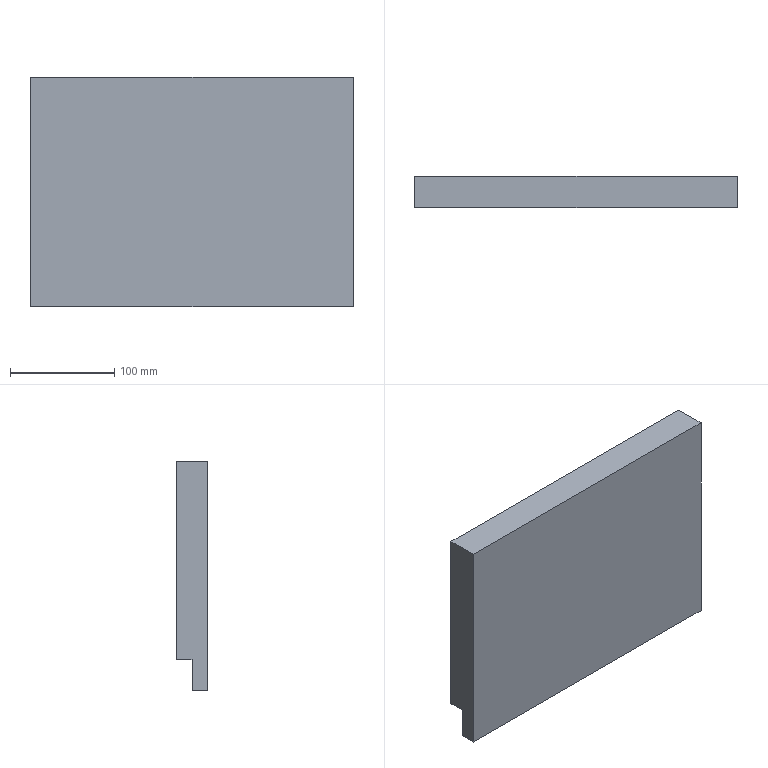Part | SolidWorks | features Cut 1, Extrusion 1 | 1 solid | 8 faces | box 308.5 x 30 x 220 mm | volume 1897275 mm3 | plane 8
STEP:
#1=CARTESIAN_POINT('',(154.25,15.,-110.));
#2=VERTEX_POINT('',#1);
#3=CARTESIAN_POINT('',(154.25,15.,-80.));
#4=VERTEX_POINT('',#3);
#5=CARTESIAN_POINT('',(154.25,15.,110.));
#6=DIRECTION('',(0.,0.,1.));
#7=VECTOR('',#6,1000.);
#8=LINE('',#5,#7);
#9=EDGE_CURVE('',#2,#4,#8,.T.);
#10=ORIENTED_EDGE('',*,*,#9,.T.);
#11=CARTESIAN_POINT('',(154.25,30.,-80.));
#12=VERTEX_POINT('',#11);
#13=CARTESIAN_POINT('',(154.25,30.,-80.));
#14=DIRECTION('',(0.,1.,0.));
#15=VECTOR('',#14,1000.);
#16=LINE('',#13,#15);
#17=EDGE_CURVE('',#4,#12,#16,.T.);
#18=ORIENTED_EDGE('',*,*,#17,.T.);
#19=CARTESIAN_POINT('',(154.25,30.,110.));
#20=VERTEX_POINT('',#19);
#21=CARTESIAN_POINT('',(154.25,30.,110.));
#22=DIRECTION('',(0.,0.,-1.));
#23=VECTOR('',#22,1000.);
#24=LINE('',#21,#23);
#25=EDGE_CURVE('',#20,#12,#24,.T.);
#26=ORIENTED_EDGE('',*,*,#25,.F.);
#27=CARTESIAN_POINT('',(154.25,0.,110.));
#28=VERTEX_POINT('',#27);
#29=CARTESIAN_POINT('',(154.25,30.,110.));
#30=DIRECTION('',(0.,-1.,0.));
#31=VECTOR('',#30,1000.);
#32=LINE('',#29,#31);
#33=EDGE_CURVE('',#20,#28,#32,.T.);
#34=ORIENTED_EDGE('',*,*,#33,.T.);
#35=CARTESIAN_POINT('',(154.25,0.,-110.));
#36=VERTEX_POINT('',#35);
#37=CARTESIAN_POINT('',(154.25,0.,110.));
#38=DIRECTION('',(0.,0.,-1.));
#39=VECTOR('',#38,1000.);
#40=LINE('',#37,#39);
#41=EDGE_CURVE('',#28,#36,#40,.T.);
#42=ORIENTED_EDGE('',*,*,#41,.T.);
#43=CARTESIAN_POINT('',(154.25,30.,-110.));
#44=DIRECTION('',(0.,-1.,0.));
#45=VECTOR('',#44,1000.);
#46=LINE('',#43,#45);
#47=EDGE_CURVE('',#2,#36,#46,.T.);
#48=ORIENTED_EDGE('',*,*,#47,.F.);
#49=EDGE_LOOP('',(#10,#18,#26,#34,#42,#48));
#50=FACE_OUTER_BOUND('',#49,.T.);
#51=CARTESIAN_POINT('',(154.25,30.,110.));
#52=DIRECTION('',(-1.,0.,0.));
#53=DIRECTION('',(0.,0.,1.));
#54=AXIS2_PLACEMENT_3D('',#51,#52,#53);
#55=PLANE('',#54);
#56=ADVANCED_FACE('',(#50),#55,.F.);
#57=CARTESIAN_POINT('',(-154.25,15.,-110.));
#58=VERTEX_POINT('',#57);
#59=CARTESIAN_POINT('',(-154.25,0.,-110.));
#60=VERTEX_POINT('',#59);
#61=CARTESIAN_POINT('',(-154.25,30.,-110.));
#62=DIRECTION('',(0.,-1.,0.));
#63=VECTOR('',#62,1000.);
#64=LINE('',#61,#63);
#65=EDGE_CURVE('',#58,#60,#64,.T.);
#66=ORIENTED_EDGE('',*,*,#65,.F.);
#67=CARTESIAN_POINT('',(-154.25,15.,-110.));
#68=DIRECTION('',(1.,0.,0.));
#69=VECTOR('',#68,1000.);
#70=LINE('',#67,#69);
#71=EDGE_CURVE('',#58,#2,#70,.T.);
#72=ORIENTED_EDGE('',*,*,#71,.T.);
#73=ORIENTED_EDGE('',*,*,#47,.T.);
#74=CARTESIAN_POINT('',(-154.25,0.,-110.));
#75=DIRECTION('',(-1.,0.,0.));
#76=VECTOR('',#75,1000.);
#77=LINE('',#74,#76);
#78=EDGE_CURVE('',#36,#60,#77,.T.);
#79=ORIENTED_EDGE('',*,*,#78,.T.);
#80=EDGE_LOOP('',(#66,#72,#73,#79));
#81=FACE_OUTER_BOUND('',#80,.T.);
#82=CARTESIAN_POINT('',(-154.25,30.,-110.));
#83=DIRECTION('',(0.,0.,1.));
#84=DIRECTION('',(1.,0.,0.));
#85=AXIS2_PLACEMENT_3D('',#82,#83,#84);
#86=PLANE('',#85);
#87=ADVANCED_FACE('',(#81),#86,.F.);
#88=CARTESIAN_POINT('',(-154.25,30.,-80.));
#89=VERTEX_POINT('',#88);
#90=CARTESIAN_POINT('',(-154.25,30.,110.));
#91=VERTEX_POINT('',#90);
#92=CARTESIAN_POINT('',(-154.25,30.,110.));
#93=DIRECTION('',(0.,0.,1.));
#94=VECTOR('',#93,1000.);
#95=LINE('',#92,#94);
#96=EDGE_CURVE('',#89,#91,#95,.T.);
#97=ORIENTED_EDGE('',*,*,#96,.F.);
#98=CARTESIAN_POINT('',(-154.25,15.,-80.));
#99=VERTEX_POINT('',#98);
#100=CARTESIAN_POINT('',(-154.25,30.,-80.));
#101=DIRECTION('',(0.,-1.,0.));
#102=VECTOR('',#101,1000.);
#103=LINE('',#100,#102);
#104=EDGE_CURVE('',#89,#99,#103,.T.);
#105=ORIENTED_EDGE('',*,*,#104,.T.);
#106=CARTESIAN_POINT('',(-154.25,15.,110.));
#107=DIRECTION('',(0.,0.,-1.));
#108=VECTOR('',#107,1000.);
#109=LINE('',#106,#108);
#110=EDGE_CURVE('',#99,#58,#109,.T.);
#111=ORIENTED_EDGE('',*,*,#110,.T.);
#112=ORIENTED_EDGE('',*,*,#65,.T.);
#113=CARTESIAN_POINT('',(-154.25,0.,110.));
#114=VERTEX_POINT('',#113);
#115=CARTESIAN_POINT('',(-154.25,0.,110.));
#116=DIRECTION('',(0.,0.,1.));
#117=VECTOR('',#116,1000.);
#118=LINE('',#115,#117);
#119=EDGE_CURVE('',#60,#114,#118,.T.);
#120=ORIENTED_EDGE('',*,*,#119,.T.);
#121=CARTESIAN_POINT('',(-154.25,30.,110.));
#122=DIRECTION('',(0.,-1.,0.));
#123=VECTOR('',#122,1000.);
#124=LINE('',#121,#123);
#125=EDGE_CURVE('',#91,#114,#124,.T.);
#126=ORIENTED_EDGE('',*,*,#125,.F.);
#127=EDGE_LOOP('',(#97,#105,#111,#112,#120,#126));
#128=FACE_OUTER_BOUND('',#127,.T.);
#129=CARTESIAN_POINT('',(-154.25,30.,110.));
#130=DIRECTION('',(1.,0.,0.));
#131=DIRECTION('',(0.,0.,-1.));
#132=AXIS2_PLACEMENT_3D('',#129,#130,#131);
#133=PLANE('',#132);
#134=ADVANCED_FACE('',(#128),#133,.F.);
#135=CARTESIAN_POINT('',(-154.25,0.,110.));
#136=DIRECTION('',(1.,0.,0.));
#137=VECTOR('',#136,1000.);
#138=LINE('',#135,#137);
#139=EDGE_CURVE('',#114,#28,#138,.T.);
#140=ORIENTED_EDGE('',*,*,#139,.T.);
#141=ORIENTED_EDGE('',*,*,#33,.F.);
#142=CARTESIAN_POINT('',(-154.25,30.,110.));
#143=DIRECTION('',(1.,0.,0.));
#144=VECTOR('',#143,1000.);
#145=LINE('',#142,#144);
#146=EDGE_CURVE('',#91,#20,#145,.T.);
#147=ORIENTED_EDGE('',*,*,#146,.F.);
#148=ORIENTED_EDGE('',*,*,#125,.T.);
#149=EDGE_LOOP('',(#140,#141,#147,#148));
#150=FACE_OUTER_BOUND('',#149,.T.);
#151=CARTESIAN_POINT('',(-154.25,30.,110.));
#152=DIRECTION('',(0.,0.,-1.));
#153=DIRECTION('',(-1.,0.,0.));
#154=AXIS2_PLACEMENT_3D('',#151,#152,#153);
#155=PLANE('',#154);
#156=ADVANCED_FACE('',(#150),#155,.F.);
#157=ORIENTED_EDGE('',*,*,#25,.T.);
#158=CARTESIAN_POINT('',(0.,30.,-80.));
#159=DIRECTION('',(-1.,0.,0.));
#160=VECTOR('',#159,1000.);
#161=LINE('',#158,#160);
#162=EDGE_CURVE('',#12,#89,#161,.T.);
#163=ORIENTED_EDGE('',*,*,#162,.T.);
#164=ORIENTED_EDGE('',*,*,#96,.T.);
#165=ORIENTED_EDGE('',*,*,#146,.T.);
#166=EDGE_LOOP('',(#157,#163,#164,#165));
#167=FACE_OUTER_BOUND('',#166,.T.);
#168=CARTESIAN_POINT('',(0.,30.,0.));
#169=DIRECTION('',(0.,-1.,0.));
#170=DIRECTION('',(0.,0.,-1.));
#171=AXIS2_PLACEMENT_3D('',#168,#169,#170);
#172=PLANE('',#171);
#173=ADVANCED_FACE('',(#167),#172,.F.);
#174=ORIENTED_EDGE('',*,*,#41,.F.);
#175=ORIENTED_EDGE('',*,*,#139,.F.);
#176=ORIENTED_EDGE('',*,*,#119,.F.);
#177=ORIENTED_EDGE('',*,*,#78,.F.);
#178=EDGE_LOOP('',(#174,#175,#176,#177));
#179=FACE_OUTER_BOUND('',#178,.T.);
#180=CARTESIAN_POINT('',(0.,0.,0.));
#181=DIRECTION('',(0.,-1.,0.));
#182=DIRECTION('',(0.,0.,-1.));
#183=AXIS2_PLACEMENT_3D('',#180,#181,#182);
#184=PLANE('',#183);
#185=ADVANCED_FACE('',(#179),#184,.T.);
#186=ORIENTED_EDGE('',*,*,#71,.F.);
#187=ORIENTED_EDGE('',*,*,#110,.F.);
#188=CARTESIAN_POINT('',(-167.454,15.,-80.));
#189=DIRECTION('',(1.,0.,0.));
#190=VECTOR('',#189,1000.);
#191=LINE('',#188,#190);
#192=EDGE_CURVE('',#99,#4,#191,.T.);
#193=ORIENTED_EDGE('',*,*,#192,.T.);
#194=ORIENTED_EDGE('',*,*,#9,.F.);
#195=EDGE_LOOP('',(#186,#187,#193,#194));
#196=FACE_OUTER_BOUND('',#195,.T.);
#197=CARTESIAN_POINT('',(0.,15.,0.));
#198=DIRECTION('',(0.,-1.,0.));
#199=DIRECTION('',(0.,0.,-1.));
#200=AXIS2_PLACEMENT_3D('',#197,#198,#199);
#201=PLANE('',#200);
#202=ADVANCED_FACE('',(#196),#201,.F.);
#203=ORIENTED_EDGE('',*,*,#192,.F.);
#204=ORIENTED_EDGE('',*,*,#104,.F.);
#205=ORIENTED_EDGE('',*,*,#162,.F.);
#206=ORIENTED_EDGE('',*,*,#17,.F.);
#207=EDGE_LOOP('',(#203,#204,#205,#206));
#208=FACE_OUTER_BOUND('',#207,.T.);
#209=CARTESIAN_POINT('',(-167.454,15.,-80.));
#210=DIRECTION('',(0.,0.,1.));
#211=DIRECTION('',(1.,0.,0.));
#212=AXIS2_PLACEMENT_3D('',#209,#210,#211);
#213=PLANE('',#212);
#214=ADVANCED_FACE('',(#208),#213,.F.);
#215=CLOSED_SHELL('',(#56,#87,#134,#156,#173,#185,#202,#214));
#216=MANIFOLD_SOLID_BREP('',#215);
#217=CARTESIAN_POINT('',(0.,0.,0.));
#218=DIRECTION('',(0.,0.,1.));
#219=DIRECTION('',(1.,0.,0.));
#220=AXIS2_PLACEMENT_3D('',#217,#218,#219);
#221=(LENGTH_UNIT()NAMED_UNIT(*)SI_UNIT(.MILLI.,.METRE.));
#222=UNCERTAINTY_MEASURE_WITH_UNIT(LENGTH_MEASURE(0.00001),#221,'','');
#223=(NAMED_UNIT(*)PLANE_ANGLE_UNIT()SI_UNIT($,.RADIAN.));
#224=(NAMED_UNIT(*)SI_UNIT($,.STERADIAN.)SOLID_ANGLE_UNIT());
#225=(GEOMETRIC_REPRESENTATION_CONTEXT(3)GLOBAL_UNCERTAINTY_ASSIGNED_CONTEXT((#222))GLOBAL_UNIT_ASSIGNED_CONTEXT((#221,#223,#224))REPRESENTATION_CONTEXT('',''));
#226=ADVANCED_BREP_SHAPE_REPRESENTATION('',(#216,#220),#225);